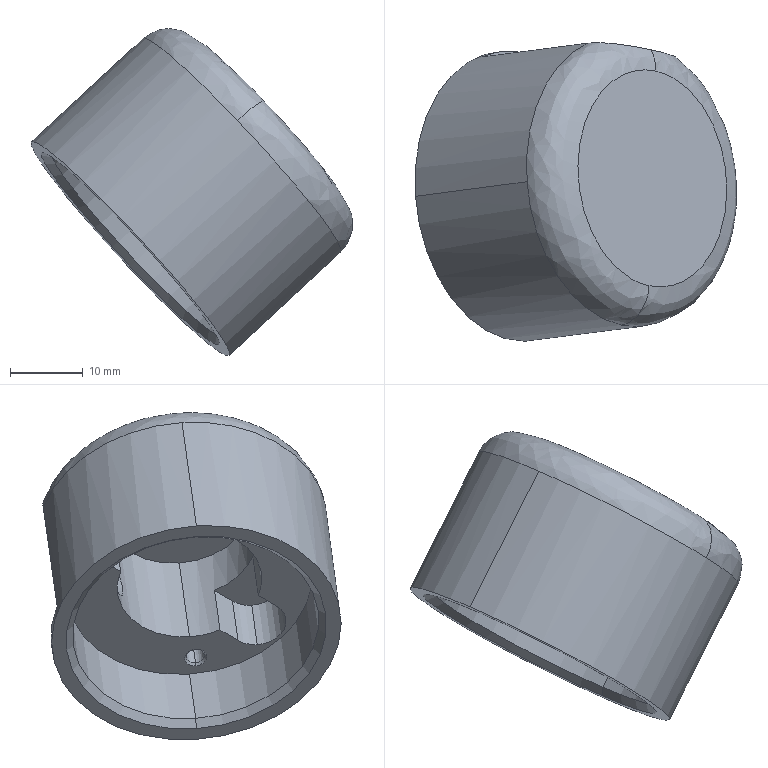Part | SolidWorks | features BaseBody 1 | 1 solid | 39 faces | box 44.241 x 41.031 x 44.985 mm | volume 16546 mm3 | cylinder 15 | plane 14 | cone 8 | spline 2 | commonest cylinder face diameters 2.5 x4 8 x3 7 x2 20 x2 34 x2 40 x2
STEP:
#1=CARTESIAN_POINT('',(719.701,-181.419,227.715));
#2=VERTEX_POINT('',#1);
#3=CARTESIAN_POINT('',(718.758,-210.958,232.869));
#4=VERTEX_POINT('',#3);
#5=CARTESIAN_POINT('',(719.701,-181.419,227.715));
#6=CARTESIAN_POINT('',(740.164,-185.821,206.224));
#7=CARTESIAN_POINT('',(739.221,-215.36,211.377));
#8=CARTESIAN_POINT('',(718.758,-210.958,232.869));
#9=(BOUNDED_CURVE()B_SPLINE_CURVE(3,(#5,#6,#7,#8),.UNSPECIFIED.,.F.,.T.)B_SPLINE_CURVE_WITH_KNOTS((4,4),(0.,1.),.UNSPECIFIED.)CURVE()GEOMETRIC_REPRESENTATION_ITEM()RATIONAL_B_SPLINE_CURVE((1.,0.3333,0.3333,1.))REPRESENTATION_ITEM(''));
#10=EDGE_CURVE('',#2,#4,#9,.T.);
#11=ORIENTED_EDGE('',*,*,#10,.T.);
#12=CARTESIAN_POINT('',(714.948,-216.354,230.346));
#13=VERTEX_POINT('',#12);
#14=CARTESIAN_POINT('',(715.105,-211.431,229.487));
#15=DIRECTION('',(0.6821,-0.1468,-0.7164));
#16=DIRECTION('',(-0.03143,-0.9846,0.1718));
#17=AXIS2_PLACEMENT_3D('',#14,#15,#16);
#18=CIRCLE('',#17,5.);
#19=EDGE_CURVE('',#4,#13,#18,.T.);
#20=ORIENTED_EDGE('',*,*,#19,.T.);
#21=CARTESIAN_POINT('',(729.162,-196.661,212.233));
#22=VERTEX_POINT('',#21);
#23=CARTESIAN_POINT('',(715.577,-196.661,226.911));
#24=DIRECTION('',(-0.7306,-0.09465,-0.6762));
#25=DIRECTION('',(0.6793,0.,-0.7339));
#26=AXIS2_PLACEMENT_3D('',#23,#24,#25);
#27=CIRCLE('',#26,20.);
#28=EDGE_CURVE('',#22,#13,#27,.T.);
#29=ORIENTED_EDGE('',*,*,#28,.F.);
#30=CARTESIAN_POINT('',(721.949,-180.088,217.706));
#31=VERTEX_POINT('',#30);
#32=CARTESIAN_POINT('',(715.577,-196.661,226.911));
#33=DIRECTION('',(-0.7306,-0.09465,-0.6762));
#34=DIRECTION('',(0.6793,0.,-0.7339));
#35=AXIS2_PLACEMENT_3D('',#32,#33,#34);
#36=CIRCLE('',#35,20.);
#37=EDGE_CURVE('',#31,#22,#36,.T.);
#38=ORIENTED_EDGE('',*,*,#37,.F.);
#39=CARTESIAN_POINT('',(719.012,-178.468,226.455));
#40=VERTEX_POINT('',#39);
#41=CARTESIAN_POINT('',(721.949,-180.088,217.706));
#42=CARTESIAN_POINT('',(722.107,-180.068,217.852));
#43=CARTESIAN_POINT('',(722.239,-180.043,218.018));
#44=CARTESIAN_POINT('',(722.454,-179.986,218.384));
#45=CARTESIAN_POINT('',(722.535,-179.954,218.582));
#46=CARTESIAN_POINT('',(722.65,-179.887,218.988));
#47=CARTESIAN_POINT('',(722.684,-179.851,219.199));
#48=CARTESIAN_POINT('',(722.713,-179.779,219.617));
#49=CARTESIAN_POINT('',(722.71,-179.743,219.826));
#50=CARTESIAN_POINT('',(722.673,-179.669,220.245));
#51=CARTESIAN_POINT('',(722.639,-179.631,220.454));
#52=CARTESIAN_POINT('',(722.551,-179.557,220.862));
#53=CARTESIAN_POINT('',(722.496,-179.52,221.063));
#54=CARTESIAN_POINT('',(722.304,-179.41,221.658));
#55=CARTESIAN_POINT('',(722.141,-179.337,222.046));
#56=CARTESIAN_POINT('',(721.584,-179.123,223.174));
#57=CARTESIAN_POINT('',(721.132,-178.987,223.872));
#58=CARTESIAN_POINT('',(720.137,-178.722,225.208));
#59=CARTESIAN_POINT('',(719.591,-178.593,225.846));
#60=CARTESIAN_POINT('',(719.012,-178.468,226.455));
#61=B_SPLINE_CURVE_WITH_KNOTS('',3,(#41,#42,#43,#44,#45,#46,#47,#48,#49,#50,#51,#52,#53,#54,#55,#56,#57,#58,#59,#60),.UNSPECIFIED.,.F.,.F.,(4,2,2,2,2,2,2,2,2,4),(0.,0.000638,0.001276,0.001914,0.002552,0.00319,0.003828,0.005104,0.007656,0.01021),.UNSPECIFIED.);
#62=EDGE_CURVE('',#31,#40,#61,.T.);
#63=ORIENTED_EDGE('',*,*,#62,.T.);
#64=CARTESIAN_POINT('',(716.048,-181.892,224.334));
#65=DIRECTION('',(-0.6821,0.1468,0.7164));
#66=DIRECTION('',(0.03143,0.9846,-0.1718));
#67=AXIS2_PLACEMENT_3D('',#64,#65,#66);
#68=CIRCLE('',#67,5.);
#69=EDGE_CURVE('',#2,#40,#68,.T.);
#70=ORIENTED_EDGE('',*,*,#69,.F.);
#71=EDGE_LOOP('',(#11,#20,#29,#38,#63,#70));
#72=FACE_OUTER_BOUND('',#71,.T.);
#73=CARTESIAN_POINT('',(718.758,-210.958,232.869));
#74=CARTESIAN_POINT('',(739.221,-215.36,211.377));
#75=CARTESIAN_POINT('',(740.164,-185.821,206.224));
#76=CARTESIAN_POINT('',(719.701,-181.419,227.715));
#77=CARTESIAN_POINT('',(718.666,-213.842,233.372));
#78=CARTESIAN_POINT('',(743.125,-219.104,207.684));
#79=CARTESIAN_POINT('',(744.252,-183.797,201.524));
#80=CARTESIAN_POINT('',(719.793,-178.535,227.212));
#81=CARTESIAN_POINT('',(717.088,-216.077,232.327));
#82=CARTESIAN_POINT('',(744.372,-221.947,203.671));
#83=CARTESIAN_POINT('',(745.629,-182.562,196.8));
#84=CARTESIAN_POINT('',(718.345,-176.691,225.456));
#85=CARTESIAN_POINT('',(714.948,-216.354,230.346));
#86=CARTESIAN_POINT('',(742.232,-222.224,201.691));
#87=CARTESIAN_POINT('',(743.489,-182.839,194.82));
#88=CARTESIAN_POINT('',(716.206,-176.969,223.475));
#89=(BOUNDED_SURFACE()B_SPLINE_SURFACE(3,3,((#73,#74,#75,#76),(#77,#78,#79,#80),(#81,#82,#83,#84),(#85,#86,#87,#88)),.UNSPECIFIED.,.F.,.F.,.F.)B_SPLINE_SURFACE_WITH_KNOTS((4,4),(4,4),(0.,1.),(0.,1.),.UNSPECIFIED.)GEOMETRIC_REPRESENTATION_ITEM()RATIONAL_B_SPLINE_SURFACE(((1.,0.3333,0.3333,1.),(0.8047,0.2682,0.2682,0.8047),(0.8047,0.2682,0.2682,0.8047),(1.,0.3333,0.3333,1.)))REPRESENTATION_ITEM('')SURFACE());
#90=ADVANCED_FACE('',(#72),#89,.T.);
#91=CARTESIAN_POINT('',(713.82,-198.649,198.032));
#92=VERTEX_POINT('',#91);
#93=CARTESIAN_POINT('',(686.649,-198.649,227.388));
#94=VERTEX_POINT('',#93);
#95=CARTESIAN_POINT('',(700.235,-198.649,212.71));
#96=DIRECTION('',(0.7306,0.09465,0.6762));
#97=DIRECTION('',(0.6793,0.,-0.7339));
#98=AXIS2_PLACEMENT_3D('',#95,#96,#97);
#99=CIRCLE('',#98,20.);
#100=EDGE_CURVE('',#92,#94,#99,.T.);
#101=ORIENTED_EDGE('',*,*,#100,.T.);
#102=CARTESIAN_POINT('',(701.991,-196.661,241.589));
#103=VERTEX_POINT('',#102);
#104=CARTESIAN_POINT('',(705.644,-196.188,244.97));
#105=DIRECTION('',(0.7306,0.09465,0.6762));
#106=VECTOR('',#105,1000.);
#107=LINE('',#104,#106);
#108=EDGE_CURVE('',#94,#103,#107,.T.);
#109=ORIENTED_EDGE('',*,*,#108,.T.);
#110=CARTESIAN_POINT('',(710.342,-177.591,229.897));
#111=VERTEX_POINT('',#110);
#112=CARTESIAN_POINT('',(715.577,-196.661,226.911));
#113=DIRECTION('',(-0.7306,-0.09465,-0.6762));
#114=DIRECTION('',(0.6793,0.,-0.7339));
#115=AXIS2_PLACEMENT_3D('',#112,#113,#114);
#116=CIRCLE('',#115,20.);
#117=EDGE_CURVE('',#103,#111,#116,.T.);
#118=ORIENTED_EDGE('',*,*,#117,.T.);
#119=CARTESIAN_POINT('',(695.731,-179.484,216.373));
#120=VERTEX_POINT('',#119);
#121=CARTESIAN_POINT('',(710.342,-177.591,229.897));
#122=DIRECTION('',(-0.7306,-0.09465,-0.6762));
#123=VECTOR('',#122,1000.);
#124=LINE('',#121,#123);
#125=EDGE_CURVE('',#111,#120,#124,.T.);
#126=ORIENTED_EDGE('',*,*,#125,.T.);
#127=CARTESIAN_POINT('',(707.338,-181.981,204.182));
#128=VERTEX_POINT('',#127);
#129=CARTESIAN_POINT('',(700.965,-198.554,213.386));
#130=DIRECTION('',(-0.7306,-0.09465,-0.6762));
#131=DIRECTION('',(0.6793,0.,-0.7339));
#132=AXIS2_PLACEMENT_3D('',#129,#130,#131);
#133=CIRCLE('',#132,20.);
#134=EDGE_CURVE('',#120,#128,#133,.T.);
#135=ORIENTED_EDGE('',*,*,#134,.T.);
#136=CARTESIAN_POINT('',(725.602,-179.615,221.087));
#137=DIRECTION('',(0.7306,0.09465,0.6762));
#138=VECTOR('',#137,1000.);
#139=LINE('',#136,#138);
#140=EDGE_CURVE('',#128,#31,#139,.T.);
#141=ORIENTED_EDGE('',*,*,#140,.T.);
#142=ORIENTED_EDGE('',*,*,#37,.T.);
#143=CARTESIAN_POINT('',(732.815,-196.188,215.614));
#144=DIRECTION('',(0.7306,0.09465,0.6762));
#145=VECTOR('',#144,1000.);
#146=LINE('',#143,#145);
#147=EDGE_CURVE('',#92,#22,#146,.T.);
#148=ORIENTED_EDGE('',*,*,#147,.F.);
#149=EDGE_LOOP('',(#101,#109,#118,#126,#135,#141,#142,#148));
#150=FACE_OUTER_BOUND('',#149,.T.);
#151=CARTESIAN_POINT('',(719.23,-196.188,230.292));
#152=DIRECTION('',(0.7306,0.09465,0.6762));
#153=DIRECTION('',(0.6793,0.,-0.7339));
#154=AXIS2_PLACEMENT_3D('',#151,#152,#153);
#155=CYLINDRICAL_SURFACE('',#154,20.);
#156=ADVANCED_FACE('',(#150),#155,.T.);
#157=CARTESIAN_POINT('',(711.753,-180.304,216.348));
#158=VERTEX_POINT('',#157);
#159=CARTESIAN_POINT('',(711.753,-179.101,223.244));
#160=VERTEX_POINT('',#159);
#161=CARTESIAN_POINT('',(711.753,-179.703,219.796));
#162=DIRECTION('',(0.03143,0.9846,-0.1718));
#163=DIRECTION('',(0.6821,-0.1468,-0.7164));
#164=AXIS2_PLACEMENT_3D('',#161,#162,#163);
#165=CIRCLE('',#164,3.5);
#166=EDGE_CURVE('',#158,#160,#165,.T.);
#167=ORIENTED_EDGE('',*,*,#166,.F.);
#168=CARTESIAN_POINT('',(711.762,-180.061,216.001));
#169=VERTEX_POINT('',#168);
#170=CARTESIAN_POINT('',(711.762,-180.061,216.001));
#171=DIRECTION('',(0.02223,0.5747,-0.8181));
#172=VECTOR('',#171,1000.);
#173=LINE('',#170,#172);
#174=EDGE_CURVE('',#158,#169,#173,.T.);
#175=ORIENTED_EDGE('',*,*,#174,.T.);
#176=CARTESIAN_POINT('',(711.762,-178.754,223.488));
#177=VERTEX_POINT('',#176);
#178=CARTESIAN_POINT('',(711.762,-179.407,219.744));
#179=DIRECTION('',(0.03143,0.9846,-0.1718));
#180=DIRECTION('',(0.,0.1719,0.9851));
#181=AXIS2_PLACEMENT_3D('',#178,#179,#180);
#182=CIRCLE('',#181,3.8);
#183=EDGE_CURVE('',#169,#177,#182,.T.);
#184=ORIENTED_EDGE('',*,*,#183,.T.);
#185=CARTESIAN_POINT('',(711.762,-178.754,223.488));
#186=DIRECTION('',(0.02223,0.8178,0.5751));
#187=VECTOR('',#186,1000.);
#188=LINE('',#185,#187);
#189=EDGE_CURVE('',#160,#177,#188,.T.);
#190=ORIENTED_EDGE('',*,*,#189,.F.);
#191=EDGE_LOOP('',(#167,#175,#184,#190));
#192=FACE_OUTER_BOUND('',#191,.T.);
#193=CARTESIAN_POINT('',(711.762,-179.407,219.744));
#194=DIRECTION('',(0.03143,0.9846,-0.1718));
#195=DIRECTION('',(0.,0.1719,0.9851));
#196=AXIS2_PLACEMENT_3D('',#193,#194,#195);
#197=CONICAL_SURFACE('',#196,3.8,0.7854);
#198=ADVANCED_FACE('',(#192),#197,.F.);
#199=CARTESIAN_POINT('',(712.513,-198.554,200.91));
#200=VERTEX_POINT('',#199);
#201=CARTESIAN_POINT('',(689.417,-198.554,225.862));
#202=VERTEX_POINT('',#201);
#203=CARTESIAN_POINT('',(700.965,-198.554,213.386));
#204=DIRECTION('',(-0.7306,-0.09465,-0.6762));
#205=DIRECTION('',(-0.03143,-0.9846,0.1718));
#206=AXIS2_PLACEMENT_3D('',#203,#204,#205);
#207=CIRCLE('',#206,17.);
#208=EDGE_CURVE('',#200,#202,#207,.T.);
#209=ORIENTED_EDGE('',*,*,#208,.F.);
#210=CARTESIAN_POINT('',(712.461,-198.649,199.5));
#211=VERTEX_POINT('',#210);
#212=CARTESIAN_POINT('',(712.461,-198.649,199.5));
#213=DIRECTION('',(-0.03629,-0.06693,-0.9971));
#214=VECTOR('',#213,1000.);
#215=LINE('',#212,#214);
#216=EDGE_CURVE('',#200,#211,#215,.T.);
#217=ORIENTED_EDGE('',*,*,#216,.T.);
#218=CARTESIAN_POINT('',(688.008,-198.649,225.92));
#219=VERTEX_POINT('',#218);
#220=CARTESIAN_POINT('',(700.235,-198.649,212.71));
#221=DIRECTION('',(0.7306,0.09465,0.6762));
#222=DIRECTION('',(-0.6793,0.,0.7339));
#223=AXIS2_PLACEMENT_3D('',#220,#221,#222);
#224=CIRCLE('',#223,18.);
#225=EDGE_CURVE('',#219,#211,#224,.T.);
#226=ORIENTED_EDGE('',*,*,#225,.F.);
#227=CARTESIAN_POINT('',(688.008,-198.649,225.92));
#228=DIRECTION('',(-0.9969,-0.06693,0.04077));
#229=VECTOR('',#228,1000.);
#230=LINE('',#227,#229);
#231=EDGE_CURVE('',#202,#219,#230,.T.);
#232=ORIENTED_EDGE('',*,*,#231,.F.);
#233=EDGE_LOOP('',(#209,#217,#226,#232));
#234=FACE_OUTER_BOUND('',#233,.T.);
#235=CARTESIAN_POINT('',(700.235,-198.649,212.71));
#236=DIRECTION('',(-0.7306,-0.09465,-0.6762));
#237=DIRECTION('',(-0.6793,0.,0.7339));
#238=AXIS2_PLACEMENT_3D('',#235,#236,#237);
#239=CONICAL_SURFACE('',#238,18.,0.7854);
#240=ADVANCED_FACE('',(#234),#239,.F.);
#241=CARTESIAN_POINT('',(711.497,-188.312,217.745));
#242=VERTEX_POINT('',#241);
#243=CARTESIAN_POINT('',(711.497,-187.109,224.641));
#244=VERTEX_POINT('',#243);
#245=CARTESIAN_POINT('',(711.497,-188.312,217.745));
#246=CARTESIAN_POINT('',(711.272,-188.265,217.737));
#247=CARTESIAN_POINT('',(711.048,-188.214,217.75));
#248=CARTESIAN_POINT('',(710.603,-188.108,217.821));
#249=CARTESIAN_POINT('',(710.384,-188.055,217.879));
#250=CARTESIAN_POINT('',(709.965,-187.952,218.037));
#251=CARTESIAN_POINT('',(709.763,-187.902,218.137));
#252=CARTESIAN_POINT('',(709.378,-187.81,218.382));
#253=CARTESIAN_POINT('',(709.2,-187.769,218.523));
#254=CARTESIAN_POINT('',(708.707,-187.66,219.003));
#255=CARTESIAN_POINT('',(708.448,-187.613,219.39));
#256=CARTESIAN_POINT('',(708.182,-187.574,220.032));
#257=CARTESIAN_POINT('',(708.116,-187.567,220.252));
#258=CARTESIAN_POINT('',(708.025,-187.559,220.704));
#259=CARTESIAN_POINT('',(708.002,-187.558,220.937));
#260=CARTESIAN_POINT('',(707.999,-187.561,221.398));
#261=CARTESIAN_POINT('',(708.02,-187.563,221.627));
#262=CARTESIAN_POINT('',(708.105,-187.567,222.082));
#263=CARTESIAN_POINT('',(708.171,-187.568,222.306));
#264=CARTESIAN_POINT('',(708.341,-187.563,222.732));
#265=CARTESIAN_POINT('',(708.448,-187.558,222.937));
#266=CARTESIAN_POINT('',(708.703,-187.538,223.325));
#267=CARTESIAN_POINT('',(708.849,-187.523,223.504));
#268=CARTESIAN_POINT('',(709.34,-187.463,223.994));
#269=CARTESIAN_POINT('',(709.731,-187.401,224.246));
#270=CARTESIAN_POINT('',(710.371,-187.292,224.494));
#271=CARTESIAN_POINT('',(710.59,-187.255,224.554));
#272=CARTESIAN_POINT('',(711.038,-187.18,224.63));
#273=CARTESIAN_POINT('',(711.27,-187.142,224.647));
#274=CARTESIAN_POINT('',(711.497,-187.109,224.641));
#275=B_SPLINE_CURVE_WITH_KNOTS('',3,(#245,#246,#247,#248,#249,#250,#251,#252,#253,#254,#255,#256,#257,#258,#259,#260,#261,#262,#263,#264,#265,#266,#267,#268,#269,#270,#271,#272,#273,#274),.UNSPECIFIED.,.F.,.F.,(4,2,2,2,2,2,2,2,2,2,2,2,2,2,4),(0.008147,0.008836,0.009525,0.01021,0.0109,0.01228,0.01297,0.01366,0.01435,0.01504,0.01573,0.01642,0.01779,0.01848,0.01917),.UNSPECIFIED.);
#276=EDGE_CURVE('',#242,#244,#275,.T.);
#277=ORIENTED_EDGE('',*,*,#276,.F.);
#278=CARTESIAN_POINT('',(711.605,-184.932,217.155));
#279=DIRECTION('',(0.03143,0.9846,-0.1718));
#280=VECTOR('',#279,1000.);
#281=LINE('',#278,#280);
#282=EDGE_CURVE('',#242,#158,#281,.T.);
#283=ORIENTED_EDGE('',*,*,#282,.T.);
#284=ORIENTED_EDGE('',*,*,#166,.T.);
#285=CARTESIAN_POINT('',(711.605,-183.729,224.051));
#286=DIRECTION('',(0.03143,0.9846,-0.1718));
#287=VECTOR('',#286,1000.);
#288=LINE('',#285,#287);
#289=EDGE_CURVE('',#244,#160,#288,.T.);
#290=ORIENTED_EDGE('',*,*,#289,.F.);
#291=EDGE_LOOP('',(#277,#283,#284,#290));
#292=FACE_OUTER_BOUND('',#291,.T.);
#293=CARTESIAN_POINT('',(711.605,-184.331,220.603));
#294=DIRECTION('',(0.03143,0.9846,-0.1718));
#295=DIRECTION('',(0.,0.1719,0.9851));
#296=AXIS2_PLACEMENT_3D('',#293,#294,#295);
#297=CYLINDRICAL_SURFACE('',#296,3.5);
#298=ADVANCED_FACE('',(#292),#297,.F.);
#299=CARTESIAN_POINT('',(719.088,-197.702,206.996));
#300=VERTEX_POINT('',#299);
#301=CARTESIAN_POINT('',(695.993,-197.702,231.948));
#302=VERTEX_POINT('',#301);
#303=CARTESIAN_POINT('',(707.54,-197.702,219.472));
#304=DIRECTION('',(-0.7306,-0.09465,-0.6762));
#305=DIRECTION('',(-0.6793,0.,0.7339));
#306=AXIS2_PLACEMENT_3D('',#303,#304,#305);
#307=CIRCLE('',#306,17.);
#308=EDGE_CURVE('',#300,#302,#307,.T.);
#309=ORIENTED_EDGE('',*,*,#308,.F.);
#310=CARTESIAN_POINT('',(713.974,-198.365,202.263));
#311=DIRECTION('',(-0.7306,-0.09465,-0.6762));
#312=VECTOR('',#311,1000.);
#313=LINE('',#310,#312);
#314=EDGE_CURVE('',#300,#200,#313,.T.);
#315=ORIENTED_EDGE('',*,*,#314,.T.);
#316=ORIENTED_EDGE('',*,*,#208,.T.);
#317=CARTESIAN_POINT('',(690.879,-198.365,227.215));
#318=DIRECTION('',(-0.7306,-0.09465,-0.6762));
#319=VECTOR('',#318,1000.);
#320=LINE('',#317,#319);
#321=EDGE_CURVE('',#302,#202,#320,.T.);
#322=ORIENTED_EDGE('',*,*,#321,.F.);
#323=EDGE_LOOP('',(#309,#315,#316,#322));
#324=FACE_OUTER_BOUND('',#323,.T.);
#325=CARTESIAN_POINT('',(702.426,-198.365,214.739));
#326=DIRECTION('',(-0.7306,-0.09465,-0.6762));
#327=DIRECTION('',(-0.6793,0.,0.7339));
#328=AXIS2_PLACEMENT_3D('',#325,#326,#327);
#329=CYLINDRICAL_SURFACE('',#328,17.);
#330=ADVANCED_FACE('',(#324),#329,.F.);
#331=CARTESIAN_POINT('',(725.292,-196.283,222.277));
#332=VERTEX_POINT('',#331);
#333=CARTESIAN_POINT('',(711.707,-196.283,236.955));
#334=VERTEX_POINT('',#333);
#335=CARTESIAN_POINT('',(718.499,-196.283,229.616));
#336=DIRECTION('',(-0.7306,-0.09465,-0.6762));
#337=DIRECTION('',(-0.6793,0.,0.7339));
#338=AXIS2_PLACEMENT_3D('',#335,#336,#337);
#339=CIRCLE('',#338,10.);
#340=EDGE_CURVE('',#332,#334,#339,.T.);
#341=ORIENTED_EDGE('',*,*,#340,.F.);
#342=CARTESIAN_POINT('',(714.333,-197.702,212.134));
#343=VERTEX_POINT('',#342);
#344=CARTESIAN_POINT('',(714.333,-197.702,212.134));
#345=DIRECTION('',(-0.7306,-0.09465,-0.6762));
#346=VECTOR('',#345,1000.);
#347=LINE('',#344,#346);
#348=EDGE_CURVE('',#332,#343,#347,.T.);
#349=ORIENTED_EDGE('',*,*,#348,.T.);
#350=CARTESIAN_POINT('',(713.994,-201.894,213.086));
#351=VERTEX_POINT('',#350);
#352=CARTESIAN_POINT('',(707.54,-197.702,219.472));
#353=DIRECTION('',(0.7306,0.09465,0.6762));
#354=DIRECTION('',(-0.6793,0.,0.7339));
#355=AXIS2_PLACEMENT_3D('',#352,#353,#354);
#356=CIRCLE('',#355,10.);
#357=EDGE_CURVE('',#351,#343,#356,.T.);
#358=ORIENTED_EDGE('',*,*,#357,.F.);
#359=CARTESIAN_POINT('',(719.839,-201.137,218.496));
#360=VERTEX_POINT('',#359);
#361=CARTESIAN_POINT('',(713.994,-201.894,213.086));
#362=DIRECTION('',(-0.7306,-0.09465,-0.6762));
#363=VECTOR('',#362,1000.);
#364=LINE('',#361,#363);
#365=EDGE_CURVE('',#360,#351,#364,.T.);
#366=ORIENTED_EDGE('',*,*,#365,.F.);
#367=CARTESIAN_POINT('',(716.139,-206.416,223.233));
#368=VERTEX_POINT('',#367);
#369=CARTESIAN_POINT('',(713.385,-196.945,224.882));
#370=DIRECTION('',(0.7306,0.09465,0.6762));
#371=DIRECTION('',(-0.6793,0.,0.7339));
#372=AXIS2_PLACEMENT_3D('',#369,#370,#371);
#373=CIRCLE('',#372,10.);
#374=EDGE_CURVE('',#368,#360,#373,.T.);
#375=ORIENTED_EDGE('',*,*,#374,.F.);
#376=CARTESIAN_POINT('',(710.294,-207.173,217.823));
#377=VERTEX_POINT('',#376);
#378=CARTESIAN_POINT('',(710.294,-207.173,217.823));
#379=DIRECTION('',(0.7306,0.09465,0.6762));
#380=VECTOR('',#379,1000.);
#381=LINE('',#378,#380);
#382=EDGE_CURVE('',#377,#368,#381,.T.);
#383=ORIENTED_EDGE('',*,*,#382,.F.);
#384=CARTESIAN_POINT('',(700.748,-197.702,226.811));
#385=VERTEX_POINT('',#384);
#386=CARTESIAN_POINT('',(707.54,-197.702,219.472));
#387=DIRECTION('',(0.7306,0.09465,0.6762));
#388=DIRECTION('',(-0.6793,0.,0.7339));
#389=AXIS2_PLACEMENT_3D('',#386,#387,#388);
#390=CIRCLE('',#389,10.);
#391=EDGE_CURVE('',#385,#377,#390,.T.);
#392=ORIENTED_EDGE('',*,*,#391,.F.);
#393=CARTESIAN_POINT('',(700.748,-197.702,226.811));
#394=DIRECTION('',(-0.7306,-0.09465,-0.6762));
#395=VECTOR('',#394,1000.);
#396=LINE('',#393,#395);
#397=EDGE_CURVE('',#334,#385,#396,.T.);
#398=ORIENTED_EDGE('',*,*,#397,.F.);
#399=EDGE_LOOP('',(#341,#349,#358,#366,#375,#383,#392,#398));
#400=FACE_OUTER_BOUND('',#399,.T.);
#401=CARTESIAN_POINT('',(707.54,-197.702,219.472));
#402=DIRECTION('',(-0.7306,-0.09465,-0.6762));
#403=DIRECTION('',(-0.6793,0.,0.7339));
#404=AXIS2_PLACEMENT_3D('',#401,#402,#403);
#405=CYLINDRICAL_SURFACE('',#404,10.);
#406=ADVANCED_FACE('',(#400),#405,.F.);
#407=CARTESIAN_POINT('',(699.065,-196.882,228.958));
#408=VERTEX_POINT('',#407);
#409=CARTESIAN_POINT('',(697.367,-196.882,230.792));
#410=VERTEX_POINT('',#409);
#411=CARTESIAN_POINT('',(698.216,-196.882,229.875));
#412=DIRECTION('',(-0.7306,-0.09465,-0.6762));
#413=DIRECTION('',(0.5023,-0.7453,-0.4384));
#414=AXIS2_PLACEMENT_3D('',#411,#412,#413);
#415=CIRCLE('',#414,1.25);
#416=EDGE_CURVE('',#408,#410,#415,.T.);
#417=ORIENTED_EDGE('',*,*,#416,.F.);
#418=CARTESIAN_POINT('',(699.05,-196.911,228.535));
#419=VERTEX_POINT('',#418);
#420=CARTESIAN_POINT('',(699.05,-196.911,228.535));
#421=DIRECTION('',(-0.03629,-0.06693,-0.9971));
#422=VECTOR('',#421,1000.);
#423=LINE('',#420,#422);
#424=EDGE_CURVE('',#408,#419,#423,.T.);
#425=ORIENTED_EDGE('',*,*,#424,.T.);
#426=CARTESIAN_POINT('',(696.944,-196.911,230.81));
#427=VERTEX_POINT('',#426);
#428=CARTESIAN_POINT('',(697.997,-196.911,229.672));
#429=DIRECTION('',(-0.7306,-0.09465,-0.6762));
#430=DIRECTION('',(-0.6793,0.,0.7339));
#431=AXIS2_PLACEMENT_3D('',#428,#429,#430);
#432=CIRCLE('',#431,1.55);
#433=EDGE_CURVE('',#419,#427,#432,.T.);
#434=ORIENTED_EDGE('',*,*,#433,.T.);
#435=CARTESIAN_POINT('',(696.944,-196.911,230.81));
#436=DIRECTION('',(-0.9969,-0.06693,0.04077));
#437=VECTOR('',#436,1000.);
#438=LINE('',#435,#437);
#439=EDGE_CURVE('',#410,#427,#438,.T.);
#440=ORIENTED_EDGE('',*,*,#439,.F.);
#441=EDGE_LOOP('',(#417,#425,#434,#440));
#442=FACE_OUTER_BOUND('',#441,.T.);
#443=CARTESIAN_POINT('',(697.997,-196.911,229.672));
#444=DIRECTION('',(-0.7306,-0.09465,-0.6762));
#445=DIRECTION('',(-0.6793,0.,0.7339));
#446=AXIS2_PLACEMENT_3D('',#443,#444,#445);
#447=CONICAL_SURFACE('',#446,1.55,0.7854);
#448=ADVANCED_FACE('',(#442),#447,.F.);
#449=CARTESIAN_POINT('',(718.165,-198.52,208.552));
#450=VERTEX_POINT('',#449);
#451=CARTESIAN_POINT('',(716.467,-198.52,210.386));
#452=VERTEX_POINT('',#451);
#453=CARTESIAN_POINT('',(717.316,-198.52,209.469));
#454=DIRECTION('',(-0.7306,-0.09465,-0.6762));
#455=DIRECTION('',(0.5023,-0.7453,-0.4384));
#456=AXIS2_PLACEMENT_3D('',#453,#454,#455);
#457=CIRCLE('',#456,1.25);
#458=EDGE_CURVE('',#450,#452,#457,.T.);
#459=ORIENTED_EDGE('',*,*,#458,.F.);
#460=CARTESIAN_POINT('',(718.149,-198.548,208.129));
#461=VERTEX_POINT('',#460);
#462=CARTESIAN_POINT('',(718.149,-198.548,208.129));
#463=DIRECTION('',(-0.03629,-0.06693,-0.9971));
#464=VECTOR('',#463,1000.);
#465=LINE('',#462,#464);
#466=EDGE_CURVE('',#450,#461,#465,.T.);
#467=ORIENTED_EDGE('',*,*,#466,.T.);
#468=CARTESIAN_POINT('',(716.044,-198.548,210.404));
#469=VERTEX_POINT('',#468);
#470=CARTESIAN_POINT('',(717.097,-198.548,209.266));
#471=DIRECTION('',(-0.7306,-0.09465,-0.6762));
#472=DIRECTION('',(-0.6793,0.,0.7339));
#473=AXIS2_PLACEMENT_3D('',#470,#471,#472);
#474=CIRCLE('',#473,1.55);
#475=EDGE_CURVE('',#461,#469,#474,.T.);
#476=ORIENTED_EDGE('',*,*,#475,.T.);
#477=CARTESIAN_POINT('',(716.044,-198.548,210.404));
#478=DIRECTION('',(-0.9969,-0.06693,0.04077));
#479=VECTOR('',#478,1000.);
#480=LINE('',#477,#479);
#481=EDGE_CURVE('',#452,#469,#480,.T.);
#482=ORIENTED_EDGE('',*,*,#481,.F.);
#483=EDGE_LOOP('',(#459,#467,#476,#482));
#484=FACE_OUTER_BOUND('',#483,.T.);
#485=CARTESIAN_POINT('',(717.097,-198.548,209.266));
#486=DIRECTION('',(-0.7306,-0.09465,-0.6762));
#487=DIRECTION('',(-0.6793,0.,0.7339));
#488=AXIS2_PLACEMENT_3D('',#485,#486,#487);
#489=CONICAL_SURFACE('',#488,1.55,0.7854);
#490=ADVANCED_FACE('',(#484),#489,.F.);
#491=CARTESIAN_POINT('',(715.669,-204.379,211.624));
#492=VERTEX_POINT('',#491);
#493=CARTESIAN_POINT('',(716.536,-207.019,211.057));
#494=VERTEX_POINT('',#493);
#495=CARTESIAN_POINT('',(713.819,-207.019,213.993));
#496=DIRECTION('',(-0.7306,-0.09465,-0.6762));
#497=DIRECTION('',(0.6793,0.,-0.7339));
#498=AXIS2_PLACEMENT_3D('',#495,#496,#497);
#499=CIRCLE('',#498,4.);
#500=EDGE_CURVE('',#492,#494,#499,.T.);
#501=ORIENTED_EDGE('',*,*,#500,.T.);
#502=CARTESIAN_POINT('',(722.381,-206.262,216.467));
#503=VERTEX_POINT('',#502);
#504=CARTESIAN_POINT('',(716.536,-207.019,211.057));
#505=DIRECTION('',(0.7306,0.09465,0.6762));
#506=VECTOR('',#505,1000.);
#507=LINE('',#504,#506);
#508=EDGE_CURVE('',#494,#503,#507,.T.);
#509=ORIENTED_EDGE('',*,*,#508,.T.);
#510=CARTESIAN_POINT('',(721.514,-203.622,217.034));
#511=VERTEX_POINT('',#510);
#512=CARTESIAN_POINT('',(719.664,-206.262,219.403));
#513=DIRECTION('',(0.7306,0.09465,0.6762));
#514=DIRECTION('',(0.6793,0.,-0.7339));
#515=AXIS2_PLACEMENT_3D('',#512,#513,#514);
#516=CIRCLE('',#515,4.);
#517=EDGE_CURVE('',#503,#511,#516,.T.);
#518=ORIENTED_EDGE('',*,*,#517,.T.);
#519=CARTESIAN_POINT('',(721.514,-203.622,217.034));
#520=DIRECTION('',(-0.7306,-0.09465,-0.6762));
#521=VECTOR('',#520,1000.);
#522=LINE('',#519,#521);
#523=EDGE_CURVE('',#511,#492,#522,.T.);
#524=ORIENTED_EDGE('',*,*,#523,.T.);
#525=EDGE_LOOP('',(#501,#509,#518,#524));
#526=FACE_OUTER_BOUND('',#525,.T.);
#527=CARTESIAN_POINT('',(713.819,-207.019,213.993));
#528=DIRECTION('',(0.7306,0.09465,0.6762));
#529=DIRECTION('',(0.6793,0.,-0.7339));
#530=AXIS2_PLACEMENT_3D('',#527,#528,#529);
#531=CYLINDRICAL_SURFACE('',#530,4.);
#532=ADVANCED_FACE('',(#526),#531,.F.);
#533=CARTESIAN_POINT('',(704.691,-196.154,234.165));
#534=VERTEX_POINT('',#533);
#535=CARTESIAN_POINT('',(702.993,-196.154,235.999));
#536=VERTEX_POINT('',#535);
#537=CARTESIAN_POINT('',(703.842,-196.154,235.082));
#538=DIRECTION('',(-0.7306,-0.09465,-0.6762));
#539=DIRECTION('',(-0.6793,0.,0.7339));
#540=AXIS2_PLACEMENT_3D('',#537,#538,#539);
#541=CIRCLE('',#540,1.25);
#542=EDGE_CURVE('',#534,#536,#541,.T.);
#543=ORIENTED_EDGE('',*,*,#542,.F.);
#544=CARTESIAN_POINT('',(701.769,-196.532,231.46));
#545=DIRECTION('',(-0.7306,-0.09465,-0.6762));
#546=VECTOR('',#545,1000.);
#547=LINE('',#544,#546);
#548=EDGE_CURVE('',#534,#408,#547,.T.);
#549=ORIENTED_EDGE('',*,*,#548,.T.);
#550=ORIENTED_EDGE('',*,*,#416,.T.);
#551=CARTESIAN_POINT('',(700.07,-196.532,233.294));
#552=DIRECTION('',(-0.7306,-0.09465,-0.6762));
#553=VECTOR('',#552,1000.);
#554=LINE('',#551,#553);
#555=EDGE_CURVE('',#536,#410,#554,.T.);
#556=ORIENTED_EDGE('',*,*,#555,.F.);
#557=EDGE_LOOP('',(#543,#549,#550,#556));
#558=FACE_OUTER_BOUND('',#557,.T.);
#559=CARTESIAN_POINT('',(700.919,-196.532,232.377));
#560=DIRECTION('',(-0.7306,-0.09465,-0.6762));
#561=DIRECTION('',(-0.6793,0.,0.7339));
#562=AXIS2_PLACEMENT_3D('',#559,#560,#561);
#563=CYLINDRICAL_SURFACE('',#562,1.25);
#564=ADVANCED_FACE('',(#558),#563,.F.);
#565=CARTESIAN_POINT('',(723.79,-197.791,213.759));
#566=VERTEX_POINT('',#565);
#567=CARTESIAN_POINT('',(722.092,-197.791,215.593));
#568=VERTEX_POINT('',#567);
#569=CARTESIAN_POINT('',(722.941,-197.791,214.676));
#570=DIRECTION('',(-0.7306,-0.09465,-0.6762));
#571=DIRECTION('',(-0.6793,0.,0.7339));
#572=AXIS2_PLACEMENT_3D('',#569,#570,#571);
#573=CIRCLE('',#572,1.25);
#574=EDGE_CURVE('',#566,#568,#573,.T.);
#575=ORIENTED_EDGE('',*,*,#574,.F.);
#576=CARTESIAN_POINT('',(720.868,-198.17,211.054));
#577=DIRECTION('',(-0.7306,-0.09465,-0.6762));
#578=VECTOR('',#577,1000.);
#579=LINE('',#576,#578);
#580=EDGE_CURVE('',#566,#450,#579,.T.);
#581=ORIENTED_EDGE('',*,*,#580,.T.);
#582=ORIENTED_EDGE('',*,*,#458,.T.);
#583=CARTESIAN_POINT('',(719.17,-198.17,212.889));
#584=DIRECTION('',(-0.7306,-0.09465,-0.6762));
#585=VECTOR('',#584,1000.);
#586=LINE('',#583,#585);
#587=EDGE_CURVE('',#568,#452,#586,.T.);
#588=ORIENTED_EDGE('',*,*,#587,.F.);
#589=EDGE_LOOP('',(#575,#581,#582,#588));
#590=FACE_OUTER_BOUND('',#589,.T.);
#591=CARTESIAN_POINT('',(720.019,-198.17,211.971));
#592=DIRECTION('',(-0.7306,-0.09465,-0.6762));
#593=DIRECTION('',(-0.6793,0.,0.7339));
#594=AXIS2_PLACEMENT_3D('',#591,#592,#593);
#595=CYLINDRICAL_SURFACE('',#594,1.25);
#596=ADVANCED_FACE('',(#590),#595,.F.);
#597=ORIENTED_EDGE('',*,*,#108,.F.);
#598=CARTESIAN_POINT('',(700.235,-198.649,212.71));
#599=DIRECTION('',(0.7306,0.09465,0.6762));
#600=DIRECTION('',(0.6793,0.,-0.7339));
#601=AXIS2_PLACEMENT_3D('',#598,#599,#600);
#602=CIRCLE('',#601,20.);
#603=EDGE_CURVE('',#94,#92,#602,.T.);
#604=ORIENTED_EDGE('',*,*,#603,.T.);
#605=ORIENTED_EDGE('',*,*,#147,.T.);
#606=ORIENTED_EDGE('',*,*,#28,.T.);
#607=CARTESIAN_POINT('',(715.577,-196.661,226.911));
#608=DIRECTION('',(-0.7306,-0.09465,-0.6762));
#609=DIRECTION('',(0.6793,0.,-0.7339));
#610=AXIS2_PLACEMENT_3D('',#607,#608,#609);
#611=CIRCLE('',#610,20.);
#612=EDGE_CURVE('',#13,#103,#611,.T.);
#613=ORIENTED_EDGE('',*,*,#612,.T.);
#614=EDGE_LOOP('',(#597,#604,#605,#606,#613));
#615=FACE_OUTER_BOUND('',#614,.T.);
#616=CARTESIAN_POINT('',(719.23,-196.188,230.292));
#617=DIRECTION('',(0.7306,0.09465,0.6762));
#618=DIRECTION('',(0.6793,0.,-0.7339));
#619=AXIS2_PLACEMENT_3D('',#616,#617,#618);
#620=CYLINDRICAL_SURFACE('',#619,20.);
#621=ADVANCED_FACE('',(#615),#620,.T.);
#622=ORIENTED_EDGE('',*,*,#19,.F.);
#623=CARTESIAN_POINT('',(718.758,-210.958,232.869));
#624=CARTESIAN_POINT('',(698.296,-206.555,254.36));
#625=CARTESIAN_POINT('',(699.239,-177.016,249.207));
#626=CARTESIAN_POINT('',(719.701,-181.419,227.715));
#627=(BOUNDED_CURVE()B_SPLINE_CURVE(3,(#623,#624,#625,#626),.UNSPECIFIED.,.F.,.F.)B_SPLINE_CURVE_WITH_KNOTS((4,4),(0.,1.),.UNSPECIFIED.)CURVE()GEOMETRIC_REPRESENTATION_ITEM()RATIONAL_B_SPLINE_CURVE((1.,0.3333,0.3333,1.))REPRESENTATION_ITEM(''));
#628=EDGE_CURVE('',#4,#2,#627,.T.);
#629=ORIENTED_EDGE('',*,*,#628,.T.);
#630=ORIENTED_EDGE('',*,*,#69,.T.);
#631=CARTESIAN_POINT('',(719.012,-178.468,226.455));
#632=CARTESIAN_POINT('',(718.433,-178.344,227.063));
#633=CARTESIAN_POINT('',(717.825,-178.224,227.637));
#634=CARTESIAN_POINT('',(716.537,-177.998,228.699));
#635=CARTESIAN_POINT('',(715.859,-177.89,229.19));
#636=CARTESIAN_POINT('',(714.748,-177.746,229.812));
#637=CARTESIAN_POINT('',(714.367,-177.702,229.996));
#638=CARTESIAN_POINT('',(713.573,-177.624,230.3));
#639=CARTESIAN_POINT('',(713.164,-177.59,230.418));
#640=CARTESIAN_POINT('',(712.535,-177.554,230.511));
#641=CARTESIAN_POINT('',(712.321,-177.544,230.529));
#642=CARTESIAN_POINT('',(711.894,-177.531,230.525));
#643=CARTESIAN_POINT('',(711.682,-177.528,230.505));
#644=CARTESIAN_POINT('',(711.263,-177.53,230.417));
#645=CARTESIAN_POINT('',(711.059,-177.535,230.35));
#646=CARTESIAN_POINT('',(710.68,-177.555,230.164));
#647=CARTESIAN_POINT('',(710.5,-177.57,230.043));
#648=CARTESIAN_POINT('',(710.342,-177.591,229.897));
#649=B_SPLINE_CURVE_WITH_KNOTS('',3,(#631,#632,#633,#634,#635,#636,#637,#638,#639,#640,#641,#642,#643,#644,#645,#646,#647,#648),.UNSPECIFIED.,.F.,.F.,(4,2,2,2,2,2,2,2,4),(0.01021,0.01276,0.01531,0.01659,0.01787,0.01851,0.01914,0.01978,0.02042),.UNSPECIFIED.);
#650=EDGE_CURVE('',#40,#111,#649,.T.);
#651=ORIENTED_EDGE('',*,*,#650,.T.);
#652=ORIENTED_EDGE('',*,*,#117,.F.);
#653=ORIENTED_EDGE('',*,*,#612,.F.);
#654=EDGE_LOOP('',(#622,#629,#630,#651,#652,#653));
#655=FACE_OUTER_BOUND('',#654,.T.);
#656=CARTESIAN_POINT('',(719.701,-181.419,227.715));
#657=CARTESIAN_POINT('',(699.239,-177.016,249.207));
#658=CARTESIAN_POINT('',(698.296,-206.555,254.36));
#659=CARTESIAN_POINT('',(718.758,-210.958,232.869));
#660=CARTESIAN_POINT('',(719.793,-178.535,227.212));
#661=CARTESIAN_POINT('',(695.335,-173.272,252.9));
#662=CARTESIAN_POINT('',(694.208,-208.579,259.06));
#663=CARTESIAN_POINT('',(718.666,-213.842,233.372));
#664=CARTESIAN_POINT('',(718.345,-176.691,225.456));
#665=CARTESIAN_POINT('',(691.062,-170.821,254.111));
#666=CARTESIAN_POINT('',(689.804,-210.207,260.983));
#667=CARTESIAN_POINT('',(717.088,-216.077,232.327));
#668=CARTESIAN_POINT('',(716.206,-176.969,223.475));
#669=CARTESIAN_POINT('',(688.922,-171.098,252.131));
#670=CARTESIAN_POINT('',(687.665,-210.484,259.002));
#671=CARTESIAN_POINT('',(714.948,-216.354,230.346));
#672=(BOUNDED_SURFACE()B_SPLINE_SURFACE(3,3,((#656,#657,#658,#659),(#660,#661,#662,#663),(#664,#665,#666,#667),(#668,#669,#670,#671)),.UNSPECIFIED.,.F.,.F.,.F.)B_SPLINE_SURFACE_WITH_KNOTS((4,4),(4,4),(0.,1.),(0.,1.),.UNSPECIFIED.)GEOMETRIC_REPRESENTATION_ITEM()RATIONAL_B_SPLINE_SURFACE(((1.,0.3333,0.3333,1.),(0.8047,0.2682,0.2682,0.8047),(0.8047,0.2682,0.2682,0.8047),(1.,0.3333,0.3333,1.)))REPRESENTATION_ITEM('')SURFACE());
#673=ADVANCED_FACE('',(#655),#672,.T.);
#674=CARTESIAN_POINT('',(711.762,-179.407,219.744));
#675=DIRECTION('',(0.03143,0.9846,-0.1718));
#676=DIRECTION('',(0.,0.1719,0.9851));
#677=AXIS2_PLACEMENT_3D('',#674,#675,#676);
#678=CIRCLE('',#677,3.8);
#679=EDGE_CURVE('',#177,#169,#678,.T.);
#680=ORIENTED_EDGE('',*,*,#679,.F.);
#681=ORIENTED_EDGE('',*,*,#183,.F.);
#682=EDGE_LOOP('',(#680,#681));
#683=FACE_BOUND('',#682,.T.);
#684=ORIENTED_EDGE('',*,*,#140,.F.);
#685=CARTESIAN_POINT('',(695.731,-179.484,216.373));
#686=DIRECTION('',(0.6821,-0.1468,-0.7164));
#687=VECTOR('',#686,1000.);
#688=LINE('',#685,#687);
#689=EDGE_CURVE('',#120,#128,#688,.T.);
#690=ORIENTED_EDGE('',*,*,#689,.F.);
#691=ORIENTED_EDGE('',*,*,#125,.F.);
#692=ORIENTED_EDGE('',*,*,#650,.F.);
#693=ORIENTED_EDGE('',*,*,#62,.F.);
#694=EDGE_LOOP('',(#684,#690,#691,#692,#693));
#695=FACE_OUTER_BOUND('',#694,.T.);
#696=CARTESIAN_POINT('',(713.995,-177.118,233.278));
#697=DIRECTION('',(-0.03143,-0.9846,0.1718));
#698=DIRECTION('',(0.,-0.1719,-0.9851));
#699=AXIS2_PLACEMENT_3D('',#696,#697,#698);
#700=PLANE('',#699);
#701=ADVANCED_FACE('',(#683,#695),#700,.F.);
#702=ORIENTED_EDGE('',*,*,#689,.T.);
#703=ORIENTED_EDGE('',*,*,#134,.F.);
#704=EDGE_LOOP('',(#702,#703));
#705=FACE_OUTER_BOUND('',#704,.T.);
#706=CARTESIAN_POINT('',(701.552,-180.164,210.178));
#707=DIRECTION('',(-0.7306,-0.09465,-0.6762));
#708=DIRECTION('',(-0.6793,0.,0.7339));
#709=AXIS2_PLACEMENT_3D('',#706,#707,#708);
#710=PLANE('',#709);
#711=ADVANCED_FACE('',(#705),#710,.F.);
#712=ORIENTED_EDGE('',*,*,#225,.T.);
#713=CARTESIAN_POINT('',(700.235,-198.649,212.71));
#714=DIRECTION('',(0.7306,0.09465,0.6762));
#715=DIRECTION('',(-0.6793,0.,0.7339));
#716=AXIS2_PLACEMENT_3D('',#713,#714,#715);
#717=CIRCLE('',#716,18.);
#718=EDGE_CURVE('',#211,#219,#717,.T.);
#719=ORIENTED_EDGE('',*,*,#718,.T.);
#720=EDGE_LOOP('',(#712,#719));
#721=FACE_BOUND('',#720,.T.);
#722=ORIENTED_EDGE('',*,*,#100,.F.);
#723=ORIENTED_EDGE('',*,*,#603,.F.);
#724=EDGE_LOOP('',(#722,#723));
#725=FACE_OUTER_BOUND('',#724,.T.);
#726=CARTESIAN_POINT('',(700.235,-198.649,212.71));
#727=DIRECTION('',(-0.7306,-0.09465,-0.6762));
#728=DIRECTION('',(-0.6793,0.,0.7339));
#729=AXIS2_PLACEMENT_3D('',#726,#727,#728);
#730=PLANE('',#729);
#731=ADVANCED_FACE('',(#721,#725),#730,.T.);
#732=ORIENTED_EDGE('',*,*,#10,.F.);
#733=ORIENTED_EDGE('',*,*,#628,.F.);
#734=EDGE_LOOP('',(#732,#733));
#735=FACE_OUTER_BOUND('',#734,.T.);
#736=CARTESIAN_POINT('',(719.23,-196.188,230.292));
#737=DIRECTION('',(-0.7306,-0.09465,-0.6762));
#738=DIRECTION('',(-0.6793,0.,0.7339));
#739=AXIS2_PLACEMENT_3D('',#736,#737,#738);
#740=PLANE('',#739);
#741=ADVANCED_FACE('',(#735),#740,.F.);
#742=ORIENTED_EDGE('',*,*,#174,.F.);
#743=CARTESIAN_POINT('',(711.753,-179.703,219.796));
#744=DIRECTION('',(0.03143,0.9846,-0.1718));
#745=DIRECTION('',(0.6821,-0.1468,-0.7164));
#746=AXIS2_PLACEMENT_3D('',#743,#744,#745);
#747=CIRCLE('',#746,3.5);
#748=EDGE_CURVE('',#160,#158,#747,.T.);
#749=ORIENTED_EDGE('',*,*,#748,.F.);
#750=ORIENTED_EDGE('',*,*,#189,.T.);
#751=ORIENTED_EDGE('',*,*,#679,.T.);
#752=EDGE_LOOP('',(#742,#749,#750,#751));
#753=FACE_OUTER_BOUND('',#752,.T.);
#754=CARTESIAN_POINT('',(711.762,-179.407,219.744));
#755=DIRECTION('',(0.03143,0.9846,-0.1718));
#756=DIRECTION('',(0.,0.1719,0.9851));
#757=AXIS2_PLACEMENT_3D('',#754,#755,#756);
#758=CONICAL_SURFACE('',#757,3.8,0.7854);
#759=ADVANCED_FACE('',(#753),#758,.F.);
#760=ORIENTED_EDGE('',*,*,#216,.F.);
#761=CARTESIAN_POINT('',(700.965,-198.554,213.386));
#762=DIRECTION('',(-0.7306,-0.09465,-0.6762));
#763=DIRECTION('',(-0.03143,-0.9846,0.1718));
#764=AXIS2_PLACEMENT_3D('',#761,#762,#763);
#765=CIRCLE('',#764,17.);
#766=EDGE_CURVE('',#202,#200,#765,.T.);
#767=ORIENTED_EDGE('',*,*,#766,.F.);
#768=ORIENTED_EDGE('',*,*,#231,.T.);
#769=ORIENTED_EDGE('',*,*,#718,.F.);
#770=EDGE_LOOP('',(#760,#767,#768,#769));
#771=FACE_OUTER_BOUND('',#770,.T.);
#772=CARTESIAN_POINT('',(700.235,-198.649,212.71));
#773=DIRECTION('',(-0.7306,-0.09465,-0.6762));
#774=DIRECTION('',(-0.6793,0.,0.7339));
#775=AXIS2_PLACEMENT_3D('',#772,#773,#774);
#776=CONICAL_SURFACE('',#775,18.,0.7854);
#777=ADVANCED_FACE('',(#771),#776,.F.);
#778=ORIENTED_EDGE('',*,*,#282,.F.);
#779=CARTESIAN_POINT('',(711.497,-187.109,224.641));
#780=CARTESIAN_POINT('',(711.725,-187.076,224.635));
#781=CARTESIAN_POINT('',(711.951,-187.046,224.608));
#782=CARTESIAN_POINT('',(712.402,-186.999,224.51));
#783=CARTESIAN_POINT('',(712.623,-186.982,224.44));
#784=CARTESIAN_POINT('',(713.046,-186.964,224.261));
#785=CARTESIAN_POINT('',(713.249,-186.964,224.152));
#786=CARTESIAN_POINT('',(713.637,-186.984,223.895));
#787=CARTESIAN_POINT('',(713.816,-187.004,223.75));
#788=CARTESIAN_POINT('',(714.308,-187.096,223.266));
#789=CARTESIAN_POINT('',(714.566,-187.198,222.889));
#790=CARTESIAN_POINT('',(714.827,-187.395,222.275));
#791=CARTESIAN_POINT('',(714.891,-187.466,222.066));
#792=CARTESIAN_POINT('',(714.977,-187.617,221.639));
#793=CARTESIAN_POINT('',(714.998,-187.698,221.419));
#794=CARTESIAN_POINT('',(714.996,-187.856,220.987));
#795=CARTESIAN_POINT('',(714.972,-187.934,220.772));
#796=CARTESIAN_POINT('',(714.882,-188.087,220.344));
#797=CARTESIAN_POINT('',(714.814,-188.159,220.133));
#798=CARTESIAN_POINT('',(714.639,-188.288,219.729));
#799=CARTESIAN_POINT('',(714.531,-188.346,219.533));
#800=CARTESIAN_POINT('',(714.273,-188.443,219.158));
#801=CARTESIAN_POINT('',(714.127,-188.481,218.983));
#802=CARTESIAN_POINT('',(713.635,-188.559,218.497));
#803=CARTESIAN_POINT('',(713.247,-188.562,218.234));
#804=CARTESIAN_POINT('',(712.611,-188.504,217.957));
#805=CARTESIAN_POINT('',(712.395,-188.475,217.886));
#806=CARTESIAN_POINT('',(711.951,-188.403,217.784));
#807=CARTESIAN_POINT('',(711.722,-188.359,217.753));
#808=CARTESIAN_POINT('',(711.497,-188.312,217.745));
#809=B_SPLINE_CURVE_WITH_KNOTS('',3,(#779,#780,#781,#782,#783,#784,#785,#786,#787,#788,#789,#790,#791,#792,#793,#794,#795,#796,#797,#798,#799,#800,#801,#802,#803,#804,#805,#806,#807,#808),.UNSPECIFIED.,.F.,.F.,(4,2,2,2,2,2,2,2,2,2,2,2,2,2,4),(-0.002877,-0.002188,-0.001499,-0.0008096,-0.0001206,0.001257,0.001946,0.002635,0.003324,0.004013,0.004702,0.005391,0.006769,0.007458,0.008147),.UNSPECIFIED.);
#810=EDGE_CURVE('',#244,#242,#809,.T.);
#811=ORIENTED_EDGE('',*,*,#810,.F.);
#812=ORIENTED_EDGE('',*,*,#289,.T.);
#813=ORIENTED_EDGE('',*,*,#748,.T.);
#814=EDGE_LOOP('',(#778,#811,#812,#813));
#815=FACE_OUTER_BOUND('',#814,.T.);
#816=CARTESIAN_POINT('',(711.605,-184.331,220.603));
#817=DIRECTION('',(0.03143,0.9846,-0.1718));
#818=DIRECTION('',(0.,0.1719,0.9851));
#819=AXIS2_PLACEMENT_3D('',#816,#817,#818);
#820=CYLINDRICAL_SURFACE('',#819,3.5);
#821=ADVANCED_FACE('',(#815),#820,.F.);
#822=ORIENTED_EDGE('',*,*,#314,.F.);
#823=CARTESIAN_POINT('',(707.54,-197.702,219.472));
#824=DIRECTION('',(-0.7306,-0.09465,-0.6762));
#825=DIRECTION('',(-0.6793,0.,0.7339));
#826=AXIS2_PLACEMENT_3D('',#823,#824,#825);
#827=CIRCLE('',#826,17.);
#828=EDGE_CURVE('',#302,#300,#827,.T.);
#829=ORIENTED_EDGE('',*,*,#828,.F.);
#830=ORIENTED_EDGE('',*,*,#321,.T.);
#831=ORIENTED_EDGE('',*,*,#766,.T.);
#832=EDGE_LOOP('',(#822,#829,#830,#831));
#833=FACE_OUTER_BOUND('',#832,.T.);
#834=CARTESIAN_POINT('',(702.426,-198.365,214.739));
#835=DIRECTION('',(-0.7306,-0.09465,-0.6762));
#836=DIRECTION('',(-0.6793,0.,0.7339));
#837=AXIS2_PLACEMENT_3D('',#834,#835,#836);
#838=CYLINDRICAL_SURFACE('',#837,17.);
#839=ADVANCED_FACE('',(#833),#838,.F.);
#840=ORIENTED_EDGE('',*,*,#348,.F.);
#841=CARTESIAN_POINT('',(718.499,-196.283,229.616));
#842=DIRECTION('',(-0.7306,-0.09465,-0.6762));
#843=DIRECTION('',(-0.6793,0.,0.7339));
#844=AXIS2_PLACEMENT_3D('',#841,#842,#843);
#845=CIRCLE('',#844,10.);
#846=EDGE_CURVE('',#334,#332,#845,.T.);
#847=ORIENTED_EDGE('',*,*,#846,.F.);
#848=ORIENTED_EDGE('',*,*,#397,.T.);
#849=CARTESIAN_POINT('',(701.087,-193.511,225.858));
#850=VERTEX_POINT('',#849);
#851=CARTESIAN_POINT('',(707.54,-197.702,219.472));
#852=DIRECTION('',(0.7306,0.09465,0.6762));
#853=DIRECTION('',(-0.6793,0.,0.7339));
#854=AXIS2_PLACEMENT_3D('',#851,#852,#853);
#855=CIRCLE('',#854,10.);
#856=EDGE_CURVE('',#850,#385,#855,.T.);
#857=ORIENTED_EDGE('',*,*,#856,.F.);
#858=CARTESIAN_POINT('',(706.931,-192.754,231.268));
#859=VERTEX_POINT('',#858);
#860=CARTESIAN_POINT('',(701.087,-193.511,225.858));
#861=DIRECTION('',(-0.7306,-0.09465,-0.6762));
#862=VECTOR('',#861,1000.);
#863=LINE('',#860,#862);
#864=EDGE_CURVE('',#859,#850,#863,.T.);
#865=ORIENTED_EDGE('',*,*,#864,.F.);
#866=CARTESIAN_POINT('',(710.632,-187.474,226.532));
#867=VERTEX_POINT('',#866);
#868=CARTESIAN_POINT('',(713.385,-196.945,224.882));
#869=DIRECTION('',(0.7306,0.09465,0.6762));
#870=DIRECTION('',(-0.6793,0.,0.7339));
#871=AXIS2_PLACEMENT_3D('',#868,#869,#870);
#872=CIRCLE('',#871,10.);
#873=EDGE_CURVE('',#867,#859,#872,.T.);
#874=ORIENTED_EDGE('',*,*,#873,.F.);
#875=CARTESIAN_POINT('',(704.787,-188.232,221.122));
#876=VERTEX_POINT('',#875);
#877=CARTESIAN_POINT('',(704.787,-188.232,221.122));
#878=DIRECTION('',(0.7306,0.09465,0.6762));
#879=VECTOR('',#878,1000.);
#880=LINE('',#877,#879);
#881=EDGE_CURVE('',#876,#867,#880,.T.);
#882=ORIENTED_EDGE('',*,*,#881,.F.);
#883=CARTESIAN_POINT('',(707.54,-197.702,219.472));
#884=DIRECTION('',(0.7306,0.09465,0.6762));
#885=DIRECTION('',(-0.6793,0.,0.7339));
#886=AXIS2_PLACEMENT_3D('',#883,#884,#885);
#887=CIRCLE('',#886,10.);
#888=EDGE_CURVE('',#343,#876,#887,.T.);
#889=ORIENTED_EDGE('',*,*,#888,.F.);
#890=EDGE_LOOP('',(#840,#847,#848,#857,#865,#874,#882,#889));
#891=FACE_OUTER_BOUND('',#890,.T.);
#892=ORIENTED_EDGE('',*,*,#810,.T.);
#893=ORIENTED_EDGE('',*,*,#276,.T.);
#894=EDGE_LOOP('',(#892,#893));
#895=FACE_BOUND('',#894,.T.);
#896=CARTESIAN_POINT('',(707.54,-197.702,219.472));
#897=DIRECTION('',(-0.7306,-0.09465,-0.6762));
#898=DIRECTION('',(-0.6793,0.,0.7339));
#899=AXIS2_PLACEMENT_3D('',#896,#897,#898);
#900=CYLINDRICAL_SURFACE('',#899,10.);
#901=ADVANCED_FACE('',(#891,#895),#900,.F.);
#902=CARTESIAN_POINT('',(697.997,-196.911,229.672));
#903=DIRECTION('',(-0.7306,-0.09465,-0.6762));
#904=DIRECTION('',(-0.6793,0.,0.7339));
#905=AXIS2_PLACEMENT_3D('',#902,#903,#904);
#906=CIRCLE('',#905,1.55);
#907=EDGE_CURVE('',#427,#419,#906,.T.);
#908=ORIENTED_EDGE('',*,*,#907,.F.);
#909=ORIENTED_EDGE('',*,*,#433,.F.);
#910=EDGE_LOOP('',(#908,#909));
#911=FACE_BOUND('',#910,.T.);
#912=ORIENTED_EDGE('',*,*,#828,.T.);
#913=ORIENTED_EDGE('',*,*,#308,.T.);
#914=EDGE_LOOP('',(#912,#913));
#915=FACE_OUTER_BOUND('',#914,.T.);
#916=CARTESIAN_POINT('',(717.097,-198.548,209.266));
#917=DIRECTION('',(-0.7306,-0.09465,-0.6762));
#918=DIRECTION('',(-0.6793,0.,0.7339));
#919=AXIS2_PLACEMENT_3D('',#916,#917,#918);
#920=CIRCLE('',#919,1.55);
#921=EDGE_CURVE('',#469,#461,#920,.T.);
#922=ORIENTED_EDGE('',*,*,#921,.F.);
#923=ORIENTED_EDGE('',*,*,#475,.F.);
#924=EDGE_LOOP('',(#922,#923));
#925=FACE_BOUND('',#924,.T.);
#926=ORIENTED_EDGE('',*,*,#856,.T.);
#927=ORIENTED_EDGE('',*,*,#391,.T.);
#928=CARTESIAN_POINT('',(711.969,-209.659,216.361));
#929=VERTEX_POINT('',#928);
#930=CARTESIAN_POINT('',(711.969,-209.659,216.361));
#931=DIRECTION('',(-0.5023,0.7453,0.4384));
#932=VECTOR('',#931,1000.);
#933=LINE('',#930,#932);
#934=EDGE_CURVE('',#929,#377,#933,.T.);
#935=ORIENTED_EDGE('',*,*,#934,.F.);
#936=CARTESIAN_POINT('',(713.819,-207.019,213.993));
#937=DIRECTION('',(-0.7306,-0.09465,-0.6762));
#938=DIRECTION('',(0.6793,0.,-0.7339));
#939=AXIS2_PLACEMENT_3D('',#936,#937,#938);
#940=CIRCLE('',#939,4.);
#941=EDGE_CURVE('',#494,#929,#940,.T.);
#942=ORIENTED_EDGE('',*,*,#941,.F.);
#943=ORIENTED_EDGE('',*,*,#500,.F.);
#944=CARTESIAN_POINT('',(713.994,-201.894,213.086));
#945=DIRECTION('',(0.5023,-0.7453,-0.4384));
#946=VECTOR('',#945,1000.);
#947=LINE('',#944,#946);
#948=EDGE_CURVE('',#351,#492,#947,.T.);
#949=ORIENTED_EDGE('',*,*,#948,.F.);
#950=ORIENTED_EDGE('',*,*,#357,.T.);
#951=ORIENTED_EDGE('',*,*,#888,.T.);
#952=CARTESIAN_POINT('',(703.112,-185.746,222.584));
#953=VERTEX_POINT('',#952);
#954=CARTESIAN_POINT('',(703.112,-185.746,222.584));
#955=DIRECTION('',(0.5023,-0.7453,-0.4384));
#956=VECTOR('',#955,1000.);
#957=LINE('',#954,#956);
#958=EDGE_CURVE('',#953,#876,#957,.T.);
#959=ORIENTED_EDGE('',*,*,#958,.F.);
#960=CARTESIAN_POINT('',(699.412,-191.026,227.32));
#961=VERTEX_POINT('',#960);
#962=CARTESIAN_POINT('',(701.262,-188.386,224.952));
#963=DIRECTION('',(-0.7306,-0.09465,-0.6762));
#964=DIRECTION('',(0.6793,0.,-0.7339));
#965=AXIS2_PLACEMENT_3D('',#962,#963,#964);
#966=CIRCLE('',#965,4.);
#967=EDGE_CURVE('',#961,#953,#966,.T.);
#968=ORIENTED_EDGE('',*,*,#967,.F.);
#969=CARTESIAN_POINT('',(701.087,-193.511,225.858));
#970=DIRECTION('',(-0.5023,0.7453,0.4384));
#971=VECTOR('',#970,1000.);
#972=LINE('',#969,#971);
#973=EDGE_CURVE('',#850,#961,#972,.T.);
#974=ORIENTED_EDGE('',*,*,#973,.F.);
#975=EDGE_LOOP('',(#926,#927,#935,#942,#943,#949,#950,#951,#959,#968,#974));
#976=FACE_BOUND('',#975,.T.);
#977=CARTESIAN_POINT('',(707.54,-197.702,219.472));
#978=DIRECTION('',(0.7306,0.09465,0.6762));
#979=DIRECTION('',(0.6793,0.,-0.7339));
#980=AXIS2_PLACEMENT_3D('',#977,#978,#979);
#981=PLANE('',#980);
#982=ADVANCED_FACE('',(#911,#915,#925,#976),#981,.F.);
#983=ORIENTED_EDGE('',*,*,#846,.T.);
#984=ORIENTED_EDGE('',*,*,#340,.T.);
#985=EDGE_LOOP('',(#983,#984));
#986=FACE_OUTER_BOUND('',#985,.T.);
#987=CARTESIAN_POINT('',(718.499,-196.283,229.616));
#988=DIRECTION('',(0.7306,0.09465,0.6762));
#989=DIRECTION('',(0.6793,0.,-0.7339));
#990=AXIS2_PLACEMENT_3D('',#987,#988,#989);
#991=PLANE('',#990);
#992=ADVANCED_FACE('',(#986),#991,.F.);
#993=ORIENTED_EDGE('',*,*,#365,.T.);
#994=ORIENTED_EDGE('',*,*,#948,.T.);
#995=ORIENTED_EDGE('',*,*,#523,.F.);
#996=CARTESIAN_POINT('',(719.839,-201.137,218.496));
#997=DIRECTION('',(0.5023,-0.7453,-0.4384));
#998=VECTOR('',#997,1000.);
#999=LINE('',#996,#998);
#1000=EDGE_CURVE('',#360,#511,#999,.T.);
#1001=ORIENTED_EDGE('',*,*,#1000,.F.);
#1002=EDGE_LOOP('',(#993,#994,#995,#1001));
#1003=FACE_OUTER_BOUND('',#1002,.T.);
#1004=CARTESIAN_POINT('',(713.994,-201.894,213.086));
#1005=DIRECTION('',(0.4625,0.6599,-0.5921));
#1006=DIRECTION('',(0.,0.6678,0.7443));
#1007=AXIS2_PLACEMENT_3D('',#1004,#1005,#1006);
#1008=PLANE('',#1007);
#1009=ADVANCED_FACE('',(#1003),#1008,.F.);
#1010=ORIENTED_EDGE('',*,*,#374,.T.);
#1011=ORIENTED_EDGE('',*,*,#1000,.T.);
#1012=ORIENTED_EDGE('',*,*,#517,.F.);
#1013=CARTESIAN_POINT('',(717.814,-208.902,221.771));
#1014=VERTEX_POINT('',#1013);
#1015=CARTESIAN_POINT('',(719.664,-206.262,219.403));
#1016=DIRECTION('',(0.7306,0.09465,0.6762));
#1017=DIRECTION('',(0.6793,0.,-0.7339));
#1018=AXIS2_PLACEMENT_3D('',#1015,#1016,#1017);
#1019=CIRCLE('',#1018,4.);
#1020=EDGE_CURVE('',#1014,#503,#1019,.T.);
#1021=ORIENTED_EDGE('',*,*,#1020,.F.);
#1022=CARTESIAN_POINT('',(716.139,-206.416,223.233));
#1023=DIRECTION('',(0.5023,-0.7453,-0.4384));
#1024=VECTOR('',#1023,1000.);
#1025=LINE('',#1022,#1024);
#1026=EDGE_CURVE('',#368,#1014,#1025,.T.);
#1027=ORIENTED_EDGE('',*,*,#1026,.F.);
#1028=EDGE_LOOP('',(#1010,#1011,#1012,#1021,#1027));
#1029=FACE_OUTER_BOUND('',#1028,.T.);
#1030=CARTESIAN_POINT('',(719.561,-206.11,219.492));
#1031=DIRECTION('',(0.7306,0.09465,0.6762));
#1032=DIRECTION('',(0.6793,0.,-0.7339));
#1033=AXIS2_PLACEMENT_3D('',#1030,#1031,#1032);
#1034=PLANE('',#1033);
#1035=ADVANCED_FACE('',(#1029),#1034,.F.);
#1036=CARTESIAN_POINT('',(711.969,-209.659,216.361));
#1037=DIRECTION('',(0.7306,0.09465,0.6762));
#1038=VECTOR('',#1037,1000.);
#1039=LINE('',#1036,#1038);
#1040=EDGE_CURVE('',#929,#1014,#1039,.T.);
#1041=ORIENTED_EDGE('',*,*,#1040,.F.);
#1042=ORIENTED_EDGE('',*,*,#934,.T.);
#1043=ORIENTED_EDGE('',*,*,#382,.T.);
#1044=ORIENTED_EDGE('',*,*,#1026,.T.);
#1045=EDGE_LOOP('',(#1041,#1042,#1043,#1044));
#1046=FACE_OUTER_BOUND('',#1045,.T.);
#1047=CARTESIAN_POINT('',(711.969,-209.659,216.361));
#1048=DIRECTION('',(-0.4625,-0.6599,0.5921));
#1049=DIRECTION('',(0.,-0.6678,-0.7443));
#1050=AXIS2_PLACEMENT_3D('',#1047,#1048,#1049);
#1051=PLANE('',#1050);
#1052=ADVANCED_FACE('',(#1046),#1051,.F.);
#1053=ORIENTED_EDGE('',*,*,#864,.T.);
#1054=ORIENTED_EDGE('',*,*,#973,.T.);
#1055=CARTESIAN_POINT('',(705.256,-190.268,232.73));
#1056=VERTEX_POINT('',#1055);
#1057=CARTESIAN_POINT('',(705.256,-190.268,232.73));
#1058=DIRECTION('',(-0.7306,-0.09465,-0.6762));
#1059=VECTOR('',#1058,1000.);
#1060=LINE('',#1057,#1059);
#1061=EDGE_CURVE('',#1056,#961,#1060,.T.);
#1062=ORIENTED_EDGE('',*,*,#1061,.F.);
#1063=CARTESIAN_POINT('',(706.931,-192.754,231.268));
#1064=DIRECTION('',(-0.5023,0.7453,0.4384));
#1065=VECTOR('',#1064,1000.);
#1066=LINE('',#1063,#1065);
#1067=EDGE_CURVE('',#859,#1056,#1066,.T.);
#1068=ORIENTED_EDGE('',*,*,#1067,.F.);
#1069=EDGE_LOOP('',(#1053,#1054,#1062,#1068));
#1070=FACE_OUTER_BOUND('',#1069,.T.);
#1071=CARTESIAN_POINT('',(701.087,-193.511,225.858));
#1072=DIRECTION('',(-0.4625,-0.6599,0.5921));
#1073=DIRECTION('',(0.,-0.6678,-0.7443));
#1074=AXIS2_PLACEMENT_3D('',#1071,#1072,#1073);
#1075=PLANE('',#1074);
#1076=ADVANCED_FACE('',(#1070),#1075,.F.);
#1077=CARTESIAN_POINT('',(708.956,-184.989,227.993));
#1078=VERTEX_POINT('',#1077);
#1079=CARTESIAN_POINT('',(707.106,-187.629,230.362));
#1080=DIRECTION('',(0.7306,0.09465,0.6762));
#1081=DIRECTION('',(0.6793,0.,-0.7339));
#1082=AXIS2_PLACEMENT_3D('',#1079,#1080,#1081);
#1083=CIRCLE('',#1082,4.);
#1084=EDGE_CURVE('',#1078,#1056,#1083,.T.);
#1085=ORIENTED_EDGE('',*,*,#1084,.F.);
#1086=CARTESIAN_POINT('',(710.632,-187.474,226.532));
#1087=DIRECTION('',(-0.5023,0.7453,0.4384));
#1088=VECTOR('',#1087,1000.);
#1089=LINE('',#1086,#1088);
#1090=EDGE_CURVE('',#867,#1078,#1089,.T.);
#1091=ORIENTED_EDGE('',*,*,#1090,.F.);
#1092=ORIENTED_EDGE('',*,*,#873,.T.);
#1093=ORIENTED_EDGE('',*,*,#1067,.T.);
#1094=EDGE_LOOP('',(#1085,#1091,#1092,#1093));
#1095=FACE_OUTER_BOUND('',#1094,.T.);
#1096=CARTESIAN_POINT('',(707.209,-187.781,230.272));
#1097=DIRECTION('',(0.7306,0.09465,0.6762));
#1098=DIRECTION('',(0.6793,0.,-0.7339));
#1099=AXIS2_PLACEMENT_3D('',#1096,#1097,#1098);
#1100=PLANE('',#1099);
#1101=ADVANCED_FACE('',(#1095),#1100,.F.);
#1102=CARTESIAN_POINT('',(703.112,-185.746,222.584));
#1103=DIRECTION('',(0.7306,0.09465,0.6762));
#1104=VECTOR('',#1103,1000.);
#1105=LINE('',#1102,#1104);
#1106=EDGE_CURVE('',#953,#1078,#1105,.T.);
#1107=ORIENTED_EDGE('',*,*,#1106,.F.);
#1108=ORIENTED_EDGE('',*,*,#958,.T.);
#1109=ORIENTED_EDGE('',*,*,#881,.T.);
#1110=ORIENTED_EDGE('',*,*,#1090,.T.);
#1111=EDGE_LOOP('',(#1107,#1108,#1109,#1110));
#1112=FACE_OUTER_BOUND('',#1111,.T.);
#1113=CARTESIAN_POINT('',(703.112,-185.746,222.584));
#1114=DIRECTION('',(0.4625,0.6599,-0.5921));
#1115=DIRECTION('',(0.,0.6678,0.7443));
#1116=AXIS2_PLACEMENT_3D('',#1113,#1114,#1115);
#1117=PLANE('',#1116);
#1118=ADVANCED_FACE('',(#1112),#1117,.F.);
#1119=ORIENTED_EDGE('',*,*,#424,.F.);
#1120=CARTESIAN_POINT('',(698.216,-196.882,229.875));
#1121=DIRECTION('',(-0.7306,-0.09465,-0.6762));
#1122=DIRECTION('',(0.5023,-0.7453,-0.4384));
#1123=AXIS2_PLACEMENT_3D('',#1120,#1121,#1122);
#1124=CIRCLE('',#1123,1.25);
#1125=EDGE_CURVE('',#410,#408,#1124,.T.);
#1126=ORIENTED_EDGE('',*,*,#1125,.F.);
#1127=ORIENTED_EDGE('',*,*,#439,.T.);
#1128=ORIENTED_EDGE('',*,*,#907,.T.);
#1129=EDGE_LOOP('',(#1119,#1126,#1127,#1128));
#1130=FACE_OUTER_BOUND('',#1129,.T.);
#1131=CARTESIAN_POINT('',(697.997,-196.911,229.672));
#1132=DIRECTION('',(-0.7306,-0.09465,-0.6762));
#1133=DIRECTION('',(-0.6793,0.,0.7339));
#1134=AXIS2_PLACEMENT_3D('',#1131,#1132,#1133);
#1135=CONICAL_SURFACE('',#1134,1.55,0.7854);
#1136=ADVANCED_FACE('',(#1130),#1135,.F.);
#1137=ORIENTED_EDGE('',*,*,#466,.F.);
#1138=CARTESIAN_POINT('',(717.316,-198.52,209.469));
#1139=DIRECTION('',(-0.7306,-0.09465,-0.6762));
#1140=DIRECTION('',(0.5023,-0.7453,-0.4384));
#1141=AXIS2_PLACEMENT_3D('',#1138,#1139,#1140);
#1142=CIRCLE('',#1141,1.25);
#1143=EDGE_CURVE('',#452,#450,#1142,.T.);
#1144=ORIENTED_EDGE('',*,*,#1143,.F.);
#1145=ORIENTED_EDGE('',*,*,#481,.T.);
#1146=ORIENTED_EDGE('',*,*,#921,.T.);
#1147=EDGE_LOOP('',(#1137,#1144,#1145,#1146));
#1148=FACE_OUTER_BOUND('',#1147,.T.);
#1149=CARTESIAN_POINT('',(717.097,-198.548,209.266));
#1150=DIRECTION('',(-0.7306,-0.09465,-0.6762));
#1151=DIRECTION('',(-0.6793,0.,0.7339));
#1152=AXIS2_PLACEMENT_3D('',#1149,#1150,#1151);
#1153=CONICAL_SURFACE('',#1152,1.55,0.7854);
#1154=ADVANCED_FACE('',(#1148),#1153,.F.);
#1155=ORIENTED_EDGE('',*,*,#508,.F.);
#1156=ORIENTED_EDGE('',*,*,#941,.T.);
#1157=ORIENTED_EDGE('',*,*,#1040,.T.);
#1158=ORIENTED_EDGE('',*,*,#1020,.T.);
#1159=EDGE_LOOP('',(#1155,#1156,#1157,#1158));
#1160=FACE_OUTER_BOUND('',#1159,.T.);
#1161=CARTESIAN_POINT('',(713.819,-207.019,213.993));
#1162=DIRECTION('',(0.7306,0.09465,0.6762));
#1163=DIRECTION('',(0.6793,0.,-0.7339));
#1164=AXIS2_PLACEMENT_3D('',#1161,#1162,#1163);
#1165=CYLINDRICAL_SURFACE('',#1164,4.);
#1166=ADVANCED_FACE('',(#1160),#1165,.F.);
#1167=ORIENTED_EDGE('',*,*,#967,.T.);
#1168=ORIENTED_EDGE('',*,*,#1106,.T.);
#1169=ORIENTED_EDGE('',*,*,#1084,.T.);
#1170=ORIENTED_EDGE('',*,*,#1061,.T.);
#1171=EDGE_LOOP('',(#1167,#1168,#1169,#1170));
#1172=FACE_OUTER_BOUND('',#1171,.T.);
#1173=CARTESIAN_POINT('',(701.262,-188.386,224.952));
#1174=DIRECTION('',(0.7306,0.09465,0.6762));
#1175=DIRECTION('',(0.6793,0.,-0.7339));
#1176=AXIS2_PLACEMENT_3D('',#1173,#1174,#1175);
#1177=CYLINDRICAL_SURFACE('',#1176,4.);
#1178=ADVANCED_FACE('',(#1172),#1177,.F.);
#1179=ORIENTED_EDGE('',*,*,#548,.F.);
#1180=CARTESIAN_POINT('',(703.842,-196.154,235.082));
#1181=DIRECTION('',(-0.7306,-0.09465,-0.6762));
#1182=DIRECTION('',(-0.6793,0.,0.7339));
#1183=AXIS2_PLACEMENT_3D('',#1180,#1181,#1182);
#1184=CIRCLE('',#1183,1.25);
#1185=EDGE_CURVE('',#536,#534,#1184,.T.);
#1186=ORIENTED_EDGE('',*,*,#1185,.F.);
#1187=ORIENTED_EDGE('',*,*,#555,.T.);
#1188=ORIENTED_EDGE('',*,*,#1125,.T.);
#1189=EDGE_LOOP('',(#1179,#1186,#1187,#1188));
#1190=FACE_OUTER_BOUND('',#1189,.T.);
#1191=CARTESIAN_POINT('',(700.919,-196.532,232.377));
#1192=DIRECTION('',(-0.7306,-0.09465,-0.6762));
#1193=DIRECTION('',(-0.6793,0.,0.7339));
#1194=AXIS2_PLACEMENT_3D('',#1191,#1192,#1193);
#1195=CYLINDRICAL_SURFACE('',#1194,1.25);
#1196=ADVANCED_FACE('',(#1190),#1195,.F.);
#1197=ORIENTED_EDGE('',*,*,#580,.F.);
#1198=CARTESIAN_POINT('',(722.941,-197.791,214.676));
#1199=DIRECTION('',(-0.7306,-0.09465,-0.6762));
#1200=DIRECTION('',(-0.6793,0.,0.7339));
#1201=AXIS2_PLACEMENT_3D('',#1198,#1199,#1200);
#1202=CIRCLE('',#1201,1.25);
#1203=EDGE_CURVE('',#568,#566,#1202,.T.);
#1204=ORIENTED_EDGE('',*,*,#1203,.F.);
#1205=ORIENTED_EDGE('',*,*,#587,.T.);
#1206=ORIENTED_EDGE('',*,*,#1143,.T.);
#1207=EDGE_LOOP('',(#1197,#1204,#1205,#1206));
#1208=FACE_OUTER_BOUND('',#1207,.T.);
#1209=CARTESIAN_POINT('',(720.019,-198.17,211.971));
#1210=DIRECTION('',(-0.7306,-0.09465,-0.6762));
#1211=DIRECTION('',(-0.6793,0.,0.7339));
#1212=AXIS2_PLACEMENT_3D('',#1209,#1210,#1211);
#1213=CYLINDRICAL_SURFACE('',#1212,1.25);
#1214=ADVANCED_FACE('',(#1208),#1213,.F.);
#1215=ORIENTED_EDGE('',*,*,#1185,.T.);
#1216=ORIENTED_EDGE('',*,*,#542,.T.);
#1217=EDGE_LOOP('',(#1215,#1216));
#1218=FACE_OUTER_BOUND('',#1217,.T.);
#1219=CARTESIAN_POINT('',(703.528,-195.688,235.356));
#1220=DIRECTION('',(0.7306,0.09465,0.6762));
#1221=DIRECTION('',(0.6793,0.,-0.7339));
#1222=AXIS2_PLACEMENT_3D('',#1219,#1220,#1221);
#1223=PLANE('',#1222);
#1224=ADVANCED_FACE('',(#1218),#1223,.F.);
#1225=ORIENTED_EDGE('',*,*,#1203,.T.);
#1226=ORIENTED_EDGE('',*,*,#574,.T.);
#1227=EDGE_LOOP('',(#1225,#1226));
#1228=FACE_OUTER_BOUND('',#1227,.T.);
#1229=CARTESIAN_POINT('',(722.627,-197.325,214.95));
#1230=DIRECTION('',(0.7306,0.09465,0.6762));
#1231=DIRECTION('',(0.6793,0.,-0.7339));
#1232=AXIS2_PLACEMENT_3D('',#1229,#1230,#1231);
#1233=PLANE('',#1232);
#1234=ADVANCED_FACE('',(#1228),#1233,.F.);
#1235=CLOSED_SHELL('',(#90,#156,#198,#240,#298,#330,#406,#448,#490,#532,#564,#596,#621,#673,#701,#711,#731,#741,#759,#777,#821,#839,#901,#982,#992,#1009,#1035,#1052,#1076,#1101,#1118,#1136,#1154,#1166,#1178,#1196,#1214,#1224,#1234));
#1236=MANIFOLD_SOLID_BREP('',#1235);
#1237=CARTESIAN_POINT('',(0.,0.,0.));
#1238=DIRECTION('',(0.,0.,1.));
#1239=DIRECTION('',(1.,0.,0.));
#1240=AXIS2_PLACEMENT_3D('',#1237,#1238,#1239);
#1241=(LENGTH_UNIT()NAMED_UNIT(*)SI_UNIT(.MILLI.,.METRE.));
#1242=UNCERTAINTY_MEASURE_WITH_UNIT(LENGTH_MEASURE(0.00001),#1241,'','');
#1243=(NAMED_UNIT(*)PLANE_ANGLE_UNIT()SI_UNIT($,.RADIAN.));
#1244=(NAMED_UNIT(*)SI_UNIT($,.STERADIAN.)SOLID_ANGLE_UNIT());
#1245=(GEOMETRIC_REPRESENTATION_CONTEXT(3)GLOBAL_UNCERTAINTY_ASSIGNED_CONTEXT((#1242))GLOBAL_UNIT_ASSIGNED_CONTEXT((#1241,#1243,#1244))REPRESENTATION_CONTEXT('',''));
#1246=ADVANCED_BREP_SHAPE_REPRESENTATION('',(#1236,#1240),#1245);